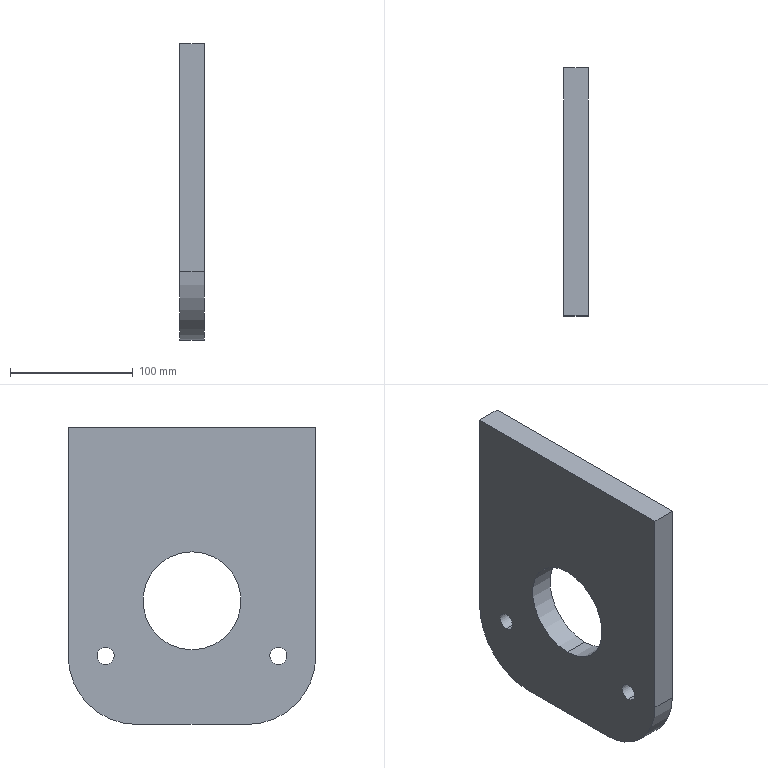Part | SolidWorks | features DeleteBody 1, MBimport 1 | 1 solid | 14 faces | box 20 x 202 x 242 mm | volume 844072 mm3 | cylinder 8 | plane 6 | commonest cylinder face diameters 14 x4 80 x2 112 x2
STEP:
#1=CARTESIAN_POINT('',(-520.5,-242.174,-1335.));
#2=VERTEX_POINT('',#1);
#3=CARTESIAN_POINT('',(-520.5,-242.174,-1349.));
#4=VERTEX_POINT('',#3);
#5=CARTESIAN_POINT('',(-520.5,-242.174,-1342.));
#6=DIRECTION('',(1.,0.,0.));
#7=DIRECTION('',(0.,1.,0.));
#8=AXIS2_PLACEMENT_3D('',#5,#6,#7);
#9=CIRCLE('',#8,7.);
#10=EDGE_CURVE('',#2,#4,#9,.T.);
#11=ORIENTED_EDGE('',*,*,#10,.F.);
#12=CARTESIAN_POINT('',(-500.5,-242.174,-1335.));
#13=VERTEX_POINT('',#12);
#14=CARTESIAN_POINT('',(-520.5,-242.174,-1335.));
#15=DIRECTION('',(1.,0.,0.));
#16=VECTOR('',#15,1000.);
#17=LINE('',#14,#16);
#18=EDGE_CURVE('',#2,#13,#17,.T.);
#19=ORIENTED_EDGE('',*,*,#18,.T.);
#20=CARTESIAN_POINT('',(-500.5,-242.174,-1349.));
#21=VERTEX_POINT('',#20);
#22=CARTESIAN_POINT('',(-500.5,-242.174,-1342.));
#23=DIRECTION('',(1.,0.,0.));
#24=DIRECTION('',(0.,1.,0.));
#25=AXIS2_PLACEMENT_3D('',#22,#23,#24);
#26=CIRCLE('',#25,7.);
#27=EDGE_CURVE('',#13,#21,#26,.T.);
#28=ORIENTED_EDGE('',*,*,#27,.T.);
#29=CARTESIAN_POINT('',(-520.5,-242.174,-1349.));
#30=DIRECTION('',(1.,0.,0.));
#31=VECTOR('',#30,1000.);
#32=LINE('',#29,#31);
#33=EDGE_CURVE('',#4,#21,#32,.T.);
#34=ORIENTED_EDGE('',*,*,#33,.F.);
#35=EDGE_LOOP('',(#11,#19,#28,#34));
#36=FACE_OUTER_BOUND('',#35,.T.);
#37=CARTESIAN_POINT('',(-520.5,-242.174,-1342.));
#38=DIRECTION('',(1.,0.,0.));
#39=DIRECTION('',(0.,0.,-1.));
#40=AXIS2_PLACEMENT_3D('',#37,#38,#39);
#41=CYLINDRICAL_SURFACE('',#40,7.);
#42=ADVANCED_FACE('',(#36),#41,.F.);
#43=CARTESIAN_POINT('',(-520.5,-171.8,-1337.227));
#44=VERTEX_POINT('',#43);
#45=CARTESIAN_POINT('',(-520.5,-171.8,-1257.227));
#46=VERTEX_POINT('',#45);
#47=CARTESIAN_POINT('',(-520.5,-171.8,-1297.227));
#48=DIRECTION('',(-1.,0.,0.));
#49=DIRECTION('',(0.,-1.,0.));
#50=AXIS2_PLACEMENT_3D('',#47,#48,#49);
#51=CIRCLE('',#50,40.);
#52=EDGE_CURVE('',#44,#46,#51,.T.);
#53=ORIENTED_EDGE('',*,*,#52,.T.);
#54=CARTESIAN_POINT('',(-500.5,-171.8,-1257.227));
#55=VERTEX_POINT('',#54);
#56=CARTESIAN_POINT('',(-520.5,-171.8,-1257.227));
#57=DIRECTION('',(1.,0.,0.));
#58=VECTOR('',#57,1000.);
#59=LINE('',#56,#58);
#60=EDGE_CURVE('',#46,#55,#59,.T.);
#61=ORIENTED_EDGE('',*,*,#60,.T.);
#62=CARTESIAN_POINT('',(-500.5,-171.8,-1337.227));
#63=VERTEX_POINT('',#62);
#64=CARTESIAN_POINT('',(-500.5,-171.8,-1297.227));
#65=DIRECTION('',(-1.,0.,0.));
#66=DIRECTION('',(0.,-1.,0.));
#67=AXIS2_PLACEMENT_3D('',#64,#65,#66);
#68=CIRCLE('',#67,40.);
#69=EDGE_CURVE('',#63,#55,#68,.T.);
#70=ORIENTED_EDGE('',*,*,#69,.F.);
#71=CARTESIAN_POINT('',(-520.5,-171.8,-1337.227));
#72=DIRECTION('',(1.,0.,0.));
#73=VECTOR('',#72,1000.);
#74=LINE('',#71,#73);
#75=EDGE_CURVE('',#44,#63,#74,.T.);
#76=ORIENTED_EDGE('',*,*,#75,.F.);
#77=EDGE_LOOP('',(#53,#61,#70,#76));
#78=FACE_OUTER_BOUND('',#77,.T.);
#79=CARTESIAN_POINT('',(-520.5,-171.8,-1297.227));
#80=DIRECTION('',(1.,0.,0.));
#81=DIRECTION('',(0.,0.,-1.));
#82=AXIS2_PLACEMENT_3D('',#79,#80,#81);
#83=CYLINDRICAL_SURFACE('',#82,40.);
#84=ADVANCED_FACE('',(#78),#83,.F.);
#85=CARTESIAN_POINT('',(-520.5,-101.426,-1349.));
#86=VERTEX_POINT('',#85);
#87=CARTESIAN_POINT('',(-520.5,-101.426,-1335.));
#88=VERTEX_POINT('',#87);
#89=CARTESIAN_POINT('',(-520.5,-101.426,-1342.));
#90=DIRECTION('',(-1.,0.,0.));
#91=DIRECTION('',(0.,-1.,0.));
#92=AXIS2_PLACEMENT_3D('',#89,#90,#91);
#93=CIRCLE('',#92,7.);
#94=EDGE_CURVE('',#86,#88,#93,.T.);
#95=ORIENTED_EDGE('',*,*,#94,.T.);
#96=CARTESIAN_POINT('',(-500.5,-101.426,-1335.));
#97=VERTEX_POINT('',#96);
#98=CARTESIAN_POINT('',(-520.5,-101.426,-1335.));
#99=DIRECTION('',(1.,0.,0.));
#100=VECTOR('',#99,1000.);
#101=LINE('',#98,#100);
#102=EDGE_CURVE('',#88,#97,#101,.T.);
#103=ORIENTED_EDGE('',*,*,#102,.T.);
#104=CARTESIAN_POINT('',(-500.5,-101.426,-1349.));
#105=VERTEX_POINT('',#104);
#106=CARTESIAN_POINT('',(-500.5,-101.426,-1342.));
#107=DIRECTION('',(-1.,0.,0.));
#108=DIRECTION('',(0.,-1.,0.));
#109=AXIS2_PLACEMENT_3D('',#106,#107,#108);
#110=CIRCLE('',#109,7.);
#111=EDGE_CURVE('',#105,#97,#110,.T.);
#112=ORIENTED_EDGE('',*,*,#111,.F.);
#113=CARTESIAN_POINT('',(-520.5,-101.426,-1349.));
#114=DIRECTION('',(1.,0.,0.));
#115=VECTOR('',#114,1000.);
#116=LINE('',#113,#115);
#117=EDGE_CURVE('',#86,#105,#116,.T.);
#118=ORIENTED_EDGE('',*,*,#117,.F.);
#119=EDGE_LOOP('',(#95,#103,#112,#118));
#120=FACE_OUTER_BOUND('',#119,.T.);
#121=CARTESIAN_POINT('',(-520.5,-101.426,-1342.));
#122=DIRECTION('',(1.,0.,0.));
#123=DIRECTION('',(0.,0.,-1.));
#124=AXIS2_PLACEMENT_3D('',#121,#122,#123);
#125=CYLINDRICAL_SURFACE('',#124,7.);
#126=ADVANCED_FACE('',(#120),#125,.F.);
#127=ORIENTED_EDGE('',*,*,#111,.T.);
#128=CARTESIAN_POINT('',(-500.5,-101.426,-1342.));
#129=DIRECTION('',(-1.,0.,0.));
#130=DIRECTION('',(0.,-1.,0.));
#131=AXIS2_PLACEMENT_3D('',#128,#129,#130);
#132=CIRCLE('',#131,7.);
#133=EDGE_CURVE('',#97,#105,#132,.T.);
#134=ORIENTED_EDGE('',*,*,#133,.T.);
#135=EDGE_LOOP('',(#127,#134));
#136=FACE_BOUND('',#135,.T.);
#137=CARTESIAN_POINT('',(-500.5,-242.174,-1342.));
#138=DIRECTION('',(1.,0.,0.));
#139=DIRECTION('',(0.,1.,0.));
#140=AXIS2_PLACEMENT_3D('',#137,#138,#139);
#141=CIRCLE('',#140,7.);
#142=EDGE_CURVE('',#21,#13,#141,.T.);
#143=ORIENTED_EDGE('',*,*,#142,.F.);
#144=ORIENTED_EDGE('',*,*,#27,.F.);
#145=EDGE_LOOP('',(#143,#144));
#146=FACE_BOUND('',#145,.T.);
#147=ORIENTED_EDGE('',*,*,#69,.T.);
#148=CARTESIAN_POINT('',(-500.5,-171.8,-1297.227));
#149=DIRECTION('',(-1.,0.,0.));
#150=DIRECTION('',(0.,-1.,0.));
#151=AXIS2_PLACEMENT_3D('',#148,#149,#150);
#152=CIRCLE('',#151,40.);
#153=EDGE_CURVE('',#55,#63,#152,.T.);
#154=ORIENTED_EDGE('',*,*,#153,.T.);
#155=EDGE_LOOP('',(#147,#154));
#156=FACE_BOUND('',#155,.T.);
#157=CARTESIAN_POINT('',(-500.5,-272.8,-1342.));
#158=VERTEX_POINT('',#157);
#159=CARTESIAN_POINT('',(-500.5,-272.8,-1156.));
#160=VERTEX_POINT('',#159);
#161=CARTESIAN_POINT('',(-500.5,-272.8,-1342.));
#162=DIRECTION('',(0.,0.,1.));
#163=VECTOR('',#162,1000.);
#164=LINE('',#161,#163);
#165=EDGE_CURVE('',#158,#160,#164,.T.);
#166=ORIENTED_EDGE('',*,*,#165,.F.);
#167=CARTESIAN_POINT('',(-500.5,-216.8,-1398.));
#168=VERTEX_POINT('',#167);
#169=CARTESIAN_POINT('',(-500.5,-216.8,-1342.));
#170=DIRECTION('',(-1.,0.,0.));
#171=DIRECTION('',(0.,-1.,0.));
#172=AXIS2_PLACEMENT_3D('',#169,#170,#171);
#173=CIRCLE('',#172,56.);
#174=EDGE_CURVE('',#168,#158,#173,.T.);
#175=ORIENTED_EDGE('',*,*,#174,.F.);
#176=CARTESIAN_POINT('',(-500.5,-126.8,-1398.));
#177=VERTEX_POINT('',#176);
#178=CARTESIAN_POINT('',(-500.5,-126.8,-1398.));
#179=DIRECTION('',(0.,-1.,0.));
#180=VECTOR('',#179,1000.);
#181=LINE('',#178,#180);
#182=EDGE_CURVE('',#177,#168,#181,.T.);
#183=ORIENTED_EDGE('',*,*,#182,.F.);
#184=CARTESIAN_POINT('',(-500.5,-70.8,-1342.));
#185=VERTEX_POINT('',#184);
#186=CARTESIAN_POINT('',(-500.5,-126.8,-1342.));
#187=DIRECTION('',(-1.,0.,0.));
#188=DIRECTION('',(0.,-1.,0.));
#189=AXIS2_PLACEMENT_3D('',#186,#187,#188);
#190=CIRCLE('',#189,56.);
#191=EDGE_CURVE('',#185,#177,#190,.T.);
#192=ORIENTED_EDGE('',*,*,#191,.F.);
#193=CARTESIAN_POINT('',(-500.5,-70.8,-1156.));
#194=VERTEX_POINT('',#193);
#195=CARTESIAN_POINT('',(-500.5,-70.8,-1156.));
#196=DIRECTION('',(0.,0.,-1.));
#197=VECTOR('',#196,1000.);
#198=LINE('',#195,#197);
#199=EDGE_CURVE('',#194,#185,#198,.T.);
#200=ORIENTED_EDGE('',*,*,#199,.F.);
#201=CARTESIAN_POINT('',(-500.5,-272.8,-1156.));
#202=DIRECTION('',(0.,1.,0.));
#203=VECTOR('',#202,1000.);
#204=LINE('',#201,#203);
#205=EDGE_CURVE('',#160,#194,#204,.T.);
#206=ORIENTED_EDGE('',*,*,#205,.F.);
#207=EDGE_LOOP('',(#166,#175,#183,#192,#200,#206));
#208=FACE_OUTER_BOUND('',#207,.T.);
#209=CARTESIAN_POINT('',(-500.5,-126.8,-1342.));
#210=DIRECTION('',(-1.,0.,0.));
#211=DIRECTION('',(0.,0.,1.));
#212=AXIS2_PLACEMENT_3D('',#209,#210,#211);
#213=PLANE('',#212);
#214=ADVANCED_FACE('',(#136,#146,#156,#208),#213,.F.);
#215=ORIENTED_EDGE('',*,*,#94,.F.);
#216=CARTESIAN_POINT('',(-520.5,-101.426,-1342.));
#217=DIRECTION('',(-1.,0.,0.));
#218=DIRECTION('',(0.,-1.,0.));
#219=AXIS2_PLACEMENT_3D('',#216,#217,#218);
#220=CIRCLE('',#219,7.);
#221=EDGE_CURVE('',#88,#86,#220,.T.);
#222=ORIENTED_EDGE('',*,*,#221,.F.);
#223=EDGE_LOOP('',(#215,#222));
#224=FACE_BOUND('',#223,.T.);
#225=CARTESIAN_POINT('',(-520.5,-242.174,-1342.));
#226=DIRECTION('',(1.,0.,0.));
#227=DIRECTION('',(0.,1.,0.));
#228=AXIS2_PLACEMENT_3D('',#225,#226,#227);
#229=CIRCLE('',#228,7.);
#230=EDGE_CURVE('',#4,#2,#229,.T.);
#231=ORIENTED_EDGE('',*,*,#230,.T.);
#232=ORIENTED_EDGE('',*,*,#10,.T.);
#233=EDGE_LOOP('',(#231,#232));
#234=FACE_BOUND('',#233,.T.);
#235=ORIENTED_EDGE('',*,*,#52,.F.);
#236=CARTESIAN_POINT('',(-520.5,-171.8,-1297.227));
#237=DIRECTION('',(-1.,0.,0.));
#238=DIRECTION('',(0.,-1.,0.));
#239=AXIS2_PLACEMENT_3D('',#236,#237,#238);
#240=CIRCLE('',#239,40.);
#241=EDGE_CURVE('',#46,#44,#240,.T.);
#242=ORIENTED_EDGE('',*,*,#241,.F.);
#243=EDGE_LOOP('',(#235,#242));
#244=FACE_BOUND('',#243,.T.);
#245=CARTESIAN_POINT('',(-520.5,-272.8,-1342.));
#246=VERTEX_POINT('',#245);
#247=CARTESIAN_POINT('',(-520.5,-272.8,-1156.));
#248=VERTEX_POINT('',#247);
#249=CARTESIAN_POINT('',(-520.5,-272.8,-1342.));
#250=DIRECTION('',(0.,0.,1.));
#251=VECTOR('',#250,1000.);
#252=LINE('',#249,#251);
#253=EDGE_CURVE('',#246,#248,#252,.T.);
#254=ORIENTED_EDGE('',*,*,#253,.T.);
#255=CARTESIAN_POINT('',(-520.5,-70.8,-1156.));
#256=VERTEX_POINT('',#255);
#257=CARTESIAN_POINT('',(-520.5,-272.8,-1156.));
#258=DIRECTION('',(0.,1.,0.));
#259=VECTOR('',#258,1000.);
#260=LINE('',#257,#259);
#261=EDGE_CURVE('',#248,#256,#260,.T.);
#262=ORIENTED_EDGE('',*,*,#261,.T.);
#263=CARTESIAN_POINT('',(-520.5,-70.8,-1342.));
#264=VERTEX_POINT('',#263);
#265=CARTESIAN_POINT('',(-520.5,-70.8,-1156.));
#266=DIRECTION('',(0.,0.,-1.));
#267=VECTOR('',#266,1000.);
#268=LINE('',#265,#267);
#269=EDGE_CURVE('',#256,#264,#268,.T.);
#270=ORIENTED_EDGE('',*,*,#269,.T.);
#271=CARTESIAN_POINT('',(-520.5,-126.8,-1398.));
#272=VERTEX_POINT('',#271);
#273=CARTESIAN_POINT('',(-520.5,-126.8,-1342.));
#274=DIRECTION('',(-1.,0.,0.));
#275=DIRECTION('',(0.,-1.,0.));
#276=AXIS2_PLACEMENT_3D('',#273,#274,#275);
#277=CIRCLE('',#276,56.);
#278=EDGE_CURVE('',#264,#272,#277,.T.);
#279=ORIENTED_EDGE('',*,*,#278,.T.);
#280=CARTESIAN_POINT('',(-520.5,-216.8,-1398.));
#281=VERTEX_POINT('',#280);
#282=CARTESIAN_POINT('',(-520.5,-126.8,-1398.));
#283=DIRECTION('',(0.,-1.,0.));
#284=VECTOR('',#283,1000.);
#285=LINE('',#282,#284);
#286=EDGE_CURVE('',#272,#281,#285,.T.);
#287=ORIENTED_EDGE('',*,*,#286,.T.);
#288=CARTESIAN_POINT('',(-520.5,-216.8,-1342.));
#289=DIRECTION('',(-1.,0.,0.));
#290=DIRECTION('',(0.,-1.,0.));
#291=AXIS2_PLACEMENT_3D('',#288,#289,#290);
#292=CIRCLE('',#291,56.);
#293=EDGE_CURVE('',#281,#246,#292,.T.);
#294=ORIENTED_EDGE('',*,*,#293,.T.);
#295=EDGE_LOOP('',(#254,#262,#270,#279,#287,#294));
#296=FACE_OUTER_BOUND('',#295,.T.);
#297=CARTESIAN_POINT('',(-520.5,-126.8,-1342.));
#298=DIRECTION('',(-1.,0.,0.));
#299=DIRECTION('',(0.,0.,1.));
#300=AXIS2_PLACEMENT_3D('',#297,#298,#299);
#301=PLANE('',#300);
#302=ADVANCED_FACE('',(#224,#234,#244,#296),#301,.T.);
#303=ORIENTED_EDGE('',*,*,#102,.F.);
#304=ORIENTED_EDGE('',*,*,#221,.T.);
#305=ORIENTED_EDGE('',*,*,#117,.T.);
#306=ORIENTED_EDGE('',*,*,#133,.F.);
#307=EDGE_LOOP('',(#303,#304,#305,#306));
#308=FACE_OUTER_BOUND('',#307,.T.);
#309=CARTESIAN_POINT('',(-520.5,-101.426,-1342.));
#310=DIRECTION('',(1.,0.,0.));
#311=DIRECTION('',(0.,0.,-1.));
#312=AXIS2_PLACEMENT_3D('',#309,#310,#311);
#313=CYLINDRICAL_SURFACE('',#312,7.);
#314=ADVANCED_FACE('',(#308),#313,.F.);
#315=ORIENTED_EDGE('',*,*,#174,.T.);
#316=CARTESIAN_POINT('',(-520.5,-272.8,-1342.));
#317=DIRECTION('',(1.,0.,0.));
#318=VECTOR('',#317,1000.);
#319=LINE('',#316,#318);
#320=EDGE_CURVE('',#246,#158,#319,.T.);
#321=ORIENTED_EDGE('',*,*,#320,.F.);
#322=ORIENTED_EDGE('',*,*,#293,.F.);
#323=CARTESIAN_POINT('',(-520.5,-216.8,-1398.));
#324=DIRECTION('',(1.,0.,0.));
#325=VECTOR('',#324,1000.);
#326=LINE('',#323,#325);
#327=EDGE_CURVE('',#281,#168,#326,.T.);
#328=ORIENTED_EDGE('',*,*,#327,.T.);
#329=EDGE_LOOP('',(#315,#321,#322,#328));
#330=FACE_OUTER_BOUND('',#329,.T.);
#331=CARTESIAN_POINT('',(-520.5,-216.8,-1342.));
#332=DIRECTION('',(1.,0.,0.));
#333=DIRECTION('',(0.,0.,-1.));
#334=AXIS2_PLACEMENT_3D('',#331,#332,#333);
#335=CYLINDRICAL_SURFACE('',#334,56.);
#336=ADVANCED_FACE('',(#330),#335,.T.);
#337=ORIENTED_EDGE('',*,*,#60,.F.);
#338=ORIENTED_EDGE('',*,*,#241,.T.);
#339=ORIENTED_EDGE('',*,*,#75,.T.);
#340=ORIENTED_EDGE('',*,*,#153,.F.);
#341=EDGE_LOOP('',(#337,#338,#339,#340));
#342=FACE_OUTER_BOUND('',#341,.T.);
#343=CARTESIAN_POINT('',(-520.5,-171.8,-1297.227));
#344=DIRECTION('',(1.,0.,0.));
#345=DIRECTION('',(0.,0.,-1.));
#346=AXIS2_PLACEMENT_3D('',#343,#344,#345);
#347=CYLINDRICAL_SURFACE('',#346,40.);
#348=ADVANCED_FACE('',(#342),#347,.F.);
#349=ORIENTED_EDGE('',*,*,#18,.F.);
#350=ORIENTED_EDGE('',*,*,#230,.F.);
#351=ORIENTED_EDGE('',*,*,#33,.T.);
#352=ORIENTED_EDGE('',*,*,#142,.T.);
#353=EDGE_LOOP('',(#349,#350,#351,#352));
#354=FACE_OUTER_BOUND('',#353,.T.);
#355=CARTESIAN_POINT('',(-520.5,-242.174,-1342.));
#356=DIRECTION('',(1.,0.,0.));
#357=DIRECTION('',(0.,0.,-1.));
#358=AXIS2_PLACEMENT_3D('',#355,#356,#357);
#359=CYLINDRICAL_SURFACE('',#358,7.);
#360=ADVANCED_FACE('',(#354),#359,.F.);
#361=ORIENTED_EDGE('',*,*,#182,.T.);
#362=ORIENTED_EDGE('',*,*,#327,.F.);
#363=ORIENTED_EDGE('',*,*,#286,.F.);
#364=CARTESIAN_POINT('',(-520.5,-126.8,-1398.));
#365=DIRECTION('',(1.,0.,0.));
#366=VECTOR('',#365,1000.);
#367=LINE('',#364,#366);
#368=EDGE_CURVE('',#272,#177,#367,.T.);
#369=ORIENTED_EDGE('',*,*,#368,.T.);
#370=EDGE_LOOP('',(#361,#362,#363,#369));
#371=FACE_OUTER_BOUND('',#370,.T.);
#372=CARTESIAN_POINT('',(-520.5,-126.8,-1398.));
#373=DIRECTION('',(0.,0.,1.));
#374=DIRECTION('',(0.,-1.,0.));
#375=AXIS2_PLACEMENT_3D('',#372,#373,#374);
#376=PLANE('',#375);
#377=ADVANCED_FACE('',(#371),#376,.F.);
#378=ORIENTED_EDGE('',*,*,#191,.T.);
#379=ORIENTED_EDGE('',*,*,#368,.F.);
#380=ORIENTED_EDGE('',*,*,#278,.F.);
#381=CARTESIAN_POINT('',(-520.5,-70.8,-1342.));
#382=DIRECTION('',(1.,0.,0.));
#383=VECTOR('',#382,1000.);
#384=LINE('',#381,#383);
#385=EDGE_CURVE('',#264,#185,#384,.T.);
#386=ORIENTED_EDGE('',*,*,#385,.T.);
#387=EDGE_LOOP('',(#378,#379,#380,#386));
#388=FACE_OUTER_BOUND('',#387,.T.);
#389=CARTESIAN_POINT('',(-520.5,-126.8,-1342.));
#390=DIRECTION('',(1.,0.,0.));
#391=DIRECTION('',(0.,0.,-1.));
#392=AXIS2_PLACEMENT_3D('',#389,#390,#391);
#393=CYLINDRICAL_SURFACE('',#392,56.);
#394=ADVANCED_FACE('',(#388),#393,.T.);
#395=ORIENTED_EDGE('',*,*,#199,.T.);
#396=ORIENTED_EDGE('',*,*,#385,.F.);
#397=ORIENTED_EDGE('',*,*,#269,.F.);
#398=CARTESIAN_POINT('',(-520.5,-70.8,-1156.));
#399=DIRECTION('',(1.,0.,0.));
#400=VECTOR('',#399,1000.);
#401=LINE('',#398,#400);
#402=EDGE_CURVE('',#256,#194,#401,.T.);
#403=ORIENTED_EDGE('',*,*,#402,.T.);
#404=EDGE_LOOP('',(#395,#396,#397,#403));
#405=FACE_OUTER_BOUND('',#404,.T.);
#406=CARTESIAN_POINT('',(-520.5,-70.8,-1156.));
#407=DIRECTION('',(0.,-1.,0.));
#408=DIRECTION('',(0.,0.,-1.));
#409=AXIS2_PLACEMENT_3D('',#406,#407,#408);
#410=PLANE('',#409);
#411=ADVANCED_FACE('',(#405),#410,.F.);
#412=ORIENTED_EDGE('',*,*,#205,.T.);
#413=ORIENTED_EDGE('',*,*,#402,.F.);
#414=ORIENTED_EDGE('',*,*,#261,.F.);
#415=CARTESIAN_POINT('',(-520.5,-272.8,-1156.));
#416=DIRECTION('',(1.,0.,0.));
#417=VECTOR('',#416,1000.);
#418=LINE('',#415,#417);
#419=EDGE_CURVE('',#248,#160,#418,.T.);
#420=ORIENTED_EDGE('',*,*,#419,.T.);
#421=EDGE_LOOP('',(#412,#413,#414,#420));
#422=FACE_OUTER_BOUND('',#421,.T.);
#423=CARTESIAN_POINT('',(-520.5,-272.8,-1156.));
#424=DIRECTION('',(0.,0.,-1.));
#425=DIRECTION('',(-1.,0.,0.));
#426=AXIS2_PLACEMENT_3D('',#423,#424,#425);
#427=PLANE('',#426);
#428=ADVANCED_FACE('',(#422),#427,.F.);
#429=ORIENTED_EDGE('',*,*,#165,.T.);
#430=ORIENTED_EDGE('',*,*,#419,.F.);
#431=ORIENTED_EDGE('',*,*,#253,.F.);
#432=ORIENTED_EDGE('',*,*,#320,.T.);
#433=EDGE_LOOP('',(#429,#430,#431,#432));
#434=FACE_OUTER_BOUND('',#433,.T.);
#435=CARTESIAN_POINT('',(-520.5,-272.8,-1342.));
#436=DIRECTION('',(0.,1.,0.));
#437=DIRECTION('',(1.,0.,0.));
#438=AXIS2_PLACEMENT_3D('',#435,#436,#437);
#439=PLANE('',#438);
#440=ADVANCED_FACE('',(#434),#439,.F.);
#441=CLOSED_SHELL('',(#42,#84,#126,#214,#302,#314,#336,#348,#360,#377,#394,#411,#428,#440));
#442=MANIFOLD_SOLID_BREP('',#441);
#443=CARTESIAN_POINT('',(0.,0.,0.));
#444=DIRECTION('',(0.,0.,1.));
#445=DIRECTION('',(1.,0.,0.));
#446=AXIS2_PLACEMENT_3D('',#443,#444,#445);
#447=(LENGTH_UNIT()NAMED_UNIT(*)SI_UNIT(.MILLI.,.METRE.));
#448=UNCERTAINTY_MEASURE_WITH_UNIT(LENGTH_MEASURE(0.00001),#447,'','');
#449=(NAMED_UNIT(*)PLANE_ANGLE_UNIT()SI_UNIT($,.RADIAN.));
#450=(NAMED_UNIT(*)SI_UNIT($,.STERADIAN.)SOLID_ANGLE_UNIT());
#451=(GEOMETRIC_REPRESENTATION_CONTEXT(3)GLOBAL_UNCERTAINTY_ASSIGNED_CONTEXT((#448))GLOBAL_UNIT_ASSIGNED_CONTEXT((#447,#449,#450))REPRESENTATION_CONTEXT('',''));
#452=ADVANCED_BREP_SHAPE_REPRESENTATION('',(#442,#446),#451);